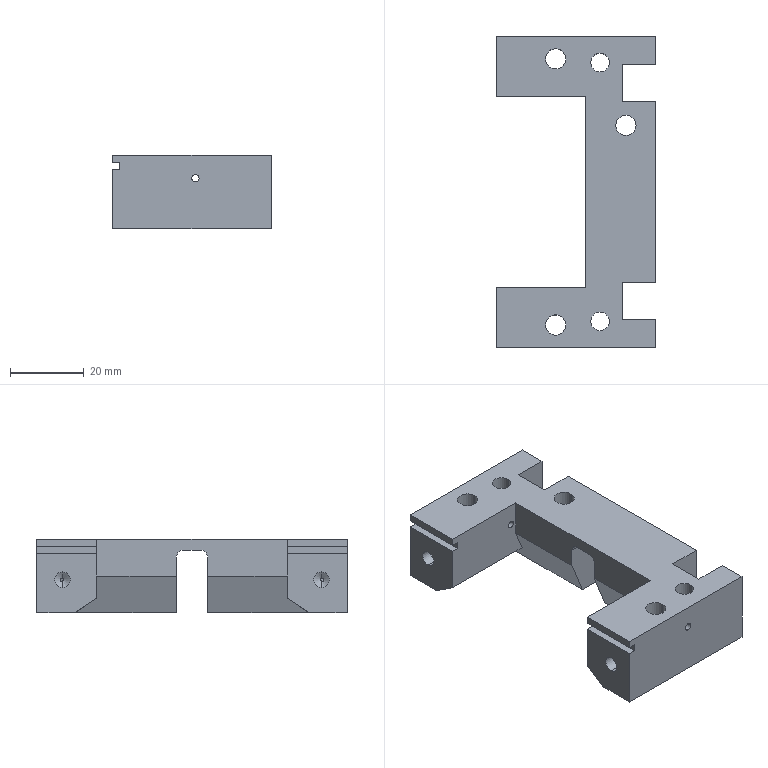Part | NX | features BREP 1 | 1 solid | 75 faces | box 43 x 84 x 20 mm | volume 35704 mm3 | plane 37 | cylinder 30 | cone 8 | commonest cylinder face diameters 5.5 x6 10 x6 2 x4 3.3 x4 4.2 x4 5 x4